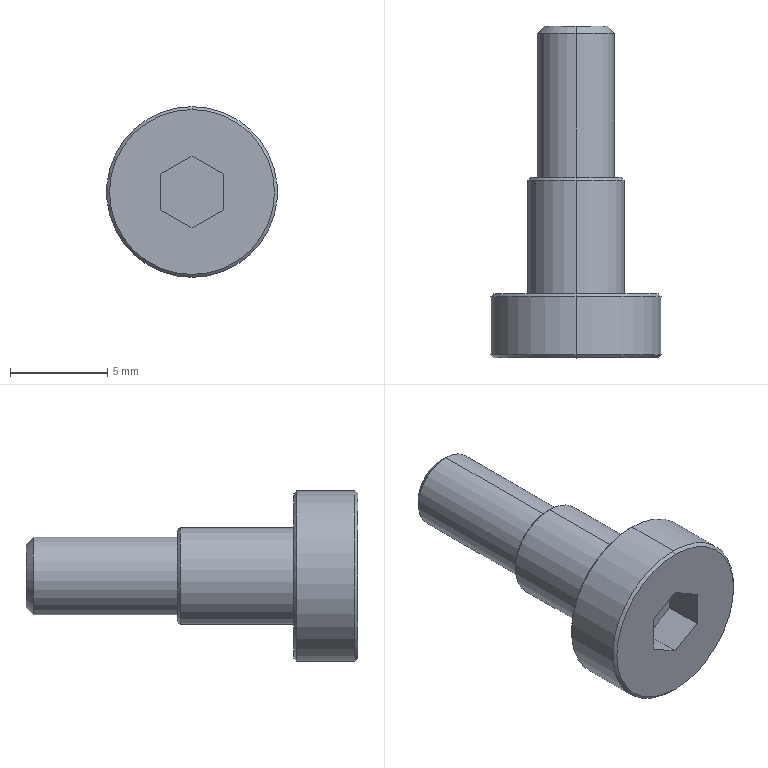Part | SolidWorks | features ICE 2, Chamfer 1, Extrusion 1, StudWizard 1 | 1 solid | 25 faces | box 8.8 x 17.1 x 8.8 mm | volume 397.168 mm3 | plane 11 | cone 8 | cylinder 6 | commonest cylinder face diameters 4 x2 5 x2 8.8 x2
STEP:
#1=CARTESIAN_POINT('',(0.,9.3,2.35));
#2=VERTEX_POINT('',#1);
#3=CARTESIAN_POINT('',(0.,9.3,-2.35));
#4=VERTEX_POINT('',#3);
#5=CARTESIAN_POINT('',(0.,9.3,0.));
#6=DIRECTION('',(0.,1.,0.));
#7=DIRECTION('',(0.,0.,1.));
#8=AXIS2_PLACEMENT_3D('',#5,#6,#7);
#9=CIRCLE('',#8,2.35);
#10=EDGE_CURVE('',#2,#4,#9,.T.);
#11=ORIENTED_EDGE('',*,*,#10,.F.);
#12=CARTESIAN_POINT('',(0.,9.15,2.5));
#13=VERTEX_POINT('',#12);
#14=CARTESIAN_POINT('',(0.,9.3,2.35));
#15=DIRECTION('',(0.,-0.7071,0.7071));
#16=VECTOR('',#15,1000.);
#17=LINE('',#14,#16);
#18=EDGE_CURVE('',#2,#13,#17,.T.);
#19=ORIENTED_EDGE('',*,*,#18,.T.);
#20=CARTESIAN_POINT('',(0.,9.15,-2.5));
#21=VERTEX_POINT('',#20);
#22=CARTESIAN_POINT('',(0.,9.15,0.));
#23=DIRECTION('',(0.,-1.,0.));
#24=DIRECTION('',(0.,0.,1.));
#25=AXIS2_PLACEMENT_3D('',#22,#23,#24);
#26=CIRCLE('',#25,2.5);
#27=EDGE_CURVE('',#21,#13,#26,.T.);
#28=ORIENTED_EDGE('',*,*,#27,.F.);
#29=CARTESIAN_POINT('',(0.,9.3,-2.35));
#30=DIRECTION('',(0.,-0.7071,-0.7071));
#31=VECTOR('',#30,1000.);
#32=LINE('',#29,#31);
#33=EDGE_CURVE('',#4,#21,#32,.T.);
#34=ORIENTED_EDGE('',*,*,#33,.F.);
#35=EDGE_LOOP('',(#11,#19,#28,#34));
#36=FACE_OUTER_BOUND('',#35,.T.);
#37=CARTESIAN_POINT('',(0.,9.3,0.));
#38=DIRECTION('',(0.,-1.,0.));
#39=DIRECTION('',(0.,0.,-1.));
#40=AXIS2_PLACEMENT_3D('',#37,#38,#39);
#41=CONICAL_SURFACE('',#40,2.35,0.7854);
#42=ADVANCED_FACE('',(#36),#41,.T.);
#43=CARTESIAN_POINT('',(0.,3.3,4.25));
#44=VERTEX_POINT('',#43);
#45=CARTESIAN_POINT('',(0.,3.3,-4.25));
#46=VERTEX_POINT('',#45);
#47=CARTESIAN_POINT('',(0.,3.3,0.));
#48=DIRECTION('',(0.,1.,0.));
#49=DIRECTION('',(0.,0.,1.));
#50=AXIS2_PLACEMENT_3D('',#47,#48,#49);
#51=CIRCLE('',#50,4.25);
#52=EDGE_CURVE('',#44,#46,#51,.T.);
#53=ORIENTED_EDGE('',*,*,#52,.F.);
#54=CARTESIAN_POINT('',(0.,3.15,4.4));
#55=VERTEX_POINT('',#54);
#56=CARTESIAN_POINT('',(0.,3.3,4.25));
#57=DIRECTION('',(0.,-0.7071,0.7071));
#58=VECTOR('',#57,1000.);
#59=LINE('',#56,#58);
#60=EDGE_CURVE('',#44,#55,#59,.T.);
#61=ORIENTED_EDGE('',*,*,#60,.T.);
#62=CARTESIAN_POINT('',(0.,3.15,-4.4));
#63=VERTEX_POINT('',#62);
#64=CARTESIAN_POINT('',(0.,3.15,0.));
#65=DIRECTION('',(0.,-1.,0.));
#66=DIRECTION('',(0.,0.,1.));
#67=AXIS2_PLACEMENT_3D('',#64,#65,#66);
#68=CIRCLE('',#67,4.4);
#69=EDGE_CURVE('',#63,#55,#68,.T.);
#70=ORIENTED_EDGE('',*,*,#69,.F.);
#71=CARTESIAN_POINT('',(0.,3.3,-4.25));
#72=DIRECTION('',(0.,-0.7071,-0.7071));
#73=VECTOR('',#72,1000.);
#74=LINE('',#71,#73);
#75=EDGE_CURVE('',#46,#63,#74,.T.);
#76=ORIENTED_EDGE('',*,*,#75,.F.);
#77=EDGE_LOOP('',(#53,#61,#70,#76));
#78=FACE_OUTER_BOUND('',#77,.T.);
#79=CARTESIAN_POINT('',(0.,3.3,0.));
#80=DIRECTION('',(0.,-1.,0.));
#81=DIRECTION('',(0.,0.,-1.));
#82=AXIS2_PLACEMENT_3D('',#79,#80,#81);
#83=CONICAL_SURFACE('',#82,4.25,0.7854);
#84=ADVANCED_FACE('',(#78),#83,.T.);
#85=CARTESIAN_POINT('',(0.,0.,-4.25));
#86=VERTEX_POINT('',#85);
#87=CARTESIAN_POINT('',(0.,0.,4.25));
#88=VERTEX_POINT('',#87);
#89=CARTESIAN_POINT('',(0.,0.,0.));
#90=DIRECTION('',(0.,-1.,0.));
#91=DIRECTION('',(0.,0.,1.));
#92=AXIS2_PLACEMENT_3D('',#89,#90,#91);
#93=CIRCLE('',#92,4.25);
#94=EDGE_CURVE('',#86,#88,#93,.T.);
#95=ORIENTED_EDGE('',*,*,#94,.F.);
#96=CARTESIAN_POINT('',(0.,0.15,-4.4));
#97=VERTEX_POINT('',#96);
#98=CARTESIAN_POINT('',(0.,0.15,-4.4));
#99=DIRECTION('',(0.,0.7071,-0.7071));
#100=VECTOR('',#99,1000.);
#101=LINE('',#98,#100);
#102=EDGE_CURVE('',#86,#97,#101,.T.);
#103=ORIENTED_EDGE('',*,*,#102,.T.);
#104=CARTESIAN_POINT('',(0.,0.15,4.4));
#105=VERTEX_POINT('',#104);
#106=CARTESIAN_POINT('',(0.,0.15,0.));
#107=DIRECTION('',(0.,1.,0.));
#108=DIRECTION('',(0.,0.,1.));
#109=AXIS2_PLACEMENT_3D('',#106,#107,#108);
#110=CIRCLE('',#109,4.4);
#111=EDGE_CURVE('',#105,#97,#110,.T.);
#112=ORIENTED_EDGE('',*,*,#111,.F.);
#113=CARTESIAN_POINT('',(0.,0.15,4.4));
#114=DIRECTION('',(0.,0.7071,0.7071));
#115=VECTOR('',#114,1000.);
#116=LINE('',#113,#115);
#117=EDGE_CURVE('',#88,#105,#116,.T.);
#118=ORIENTED_EDGE('',*,*,#117,.F.);
#119=EDGE_LOOP('',(#95,#103,#112,#118));
#120=FACE_OUTER_BOUND('',#119,.T.);
#121=CARTESIAN_POINT('',(0.,0.15,0.));
#122=DIRECTION('',(0.,1.,0.));
#123=DIRECTION('',(0.,0.,1.));
#124=AXIS2_PLACEMENT_3D('',#121,#122,#123);
#125=CONICAL_SURFACE('',#124,4.4,0.7854);
#126=ADVANCED_FACE('',(#120),#125,.T.);
#127=CARTESIAN_POINT('',(0.,16.721,-2.));
#128=VERTEX_POINT('',#127);
#129=CARTESIAN_POINT('',(0.,16.721,2.));
#130=VERTEX_POINT('',#129);
#131=CARTESIAN_POINT('',(0.,16.721,0.));
#132=DIRECTION('',(0.,-1.,0.));
#133=DIRECTION('',(0.,0.,-1.));
#134=AXIS2_PLACEMENT_3D('',#131,#132,#133);
#135=CIRCLE('',#134,2.);
#136=EDGE_CURVE('',#128,#130,#135,.T.);
#137=ORIENTED_EDGE('',*,*,#136,.T.);
#138=CARTESIAN_POINT('',(0.,9.3,2.));
#139=VERTEX_POINT('',#138);
#140=CARTESIAN_POINT('',(0.,9.3,2.));
#141=DIRECTION('',(0.,-1.,0.));
#142=VECTOR('',#141,1000.);
#143=LINE('',#140,#142);
#144=EDGE_CURVE('',#130,#139,#143,.T.);
#145=ORIENTED_EDGE('',*,*,#144,.T.);
#146=CARTESIAN_POINT('',(0.,9.3,-2.));
#147=VERTEX_POINT('',#146);
#148=CARTESIAN_POINT('',(0.,9.3,0.));
#149=DIRECTION('',(0.,-1.,0.));
#150=DIRECTION('',(0.,0.,-1.));
#151=AXIS2_PLACEMENT_3D('',#148,#149,#150);
#152=CIRCLE('',#151,2.);
#153=EDGE_CURVE('',#147,#139,#152,.T.);
#154=ORIENTED_EDGE('',*,*,#153,.F.);
#155=CARTESIAN_POINT('',(0.,9.3,-2.));
#156=DIRECTION('',(0.,-1.,0.));
#157=VECTOR('',#156,1000.);
#158=LINE('',#155,#157);
#159=EDGE_CURVE('',#128,#147,#158,.T.);
#160=ORIENTED_EDGE('',*,*,#159,.F.);
#161=EDGE_LOOP('',(#137,#145,#154,#160));
#162=FACE_OUTER_BOUND('',#161,.T.);
#163=CARTESIAN_POINT('',(0.,9.3,0.));
#164=DIRECTION('',(0.,-1.,0.));
#165=DIRECTION('',(0.,0.,-1.));
#166=AXIS2_PLACEMENT_3D('',#163,#164,#165);
#167=CYLINDRICAL_SURFACE('',#166,2.);
#168=ADVANCED_FACE('',(#162),#167,.T.);
#169=CARTESIAN_POINT('',(0.,17.1,-1.621));
#170=VERTEX_POINT('',#169);
#171=CARTESIAN_POINT('',(0.,17.1,1.621));
#172=VERTEX_POINT('',#171);
#173=CARTESIAN_POINT('',(0.,17.1,0.));
#174=DIRECTION('',(0.,-1.,0.));
#175=DIRECTION('',(0.,0.,-1.));
#176=AXIS2_PLACEMENT_3D('',#173,#174,#175);
#177=CIRCLE('',#176,1.621);
#178=EDGE_CURVE('',#170,#172,#177,.T.);
#179=ORIENTED_EDGE('',*,*,#178,.T.);
#180=CARTESIAN_POINT('',(0.,16.721,2.));
#181=DIRECTION('',(0.,-0.7071,0.7071));
#182=VECTOR('',#181,1000.);
#183=LINE('',#180,#182);
#184=EDGE_CURVE('',#172,#130,#183,.T.);
#185=ORIENTED_EDGE('',*,*,#184,.T.);
#186=ORIENTED_EDGE('',*,*,#136,.F.);
#187=CARTESIAN_POINT('',(0.,16.721,-2.));
#188=DIRECTION('',(0.,-0.7071,-0.7071));
#189=VECTOR('',#188,1000.);
#190=LINE('',#187,#189);
#191=EDGE_CURVE('',#170,#128,#190,.T.);
#192=ORIENTED_EDGE('',*,*,#191,.F.);
#193=EDGE_LOOP('',(#179,#185,#186,#192));
#194=FACE_OUTER_BOUND('',#193,.T.);
#195=CARTESIAN_POINT('',(0.,16.721,0.));
#196=DIRECTION('',(0.,-1.,0.));
#197=DIRECTION('',(0.,0.,-1.));
#198=AXIS2_PLACEMENT_3D('',#195,#196,#197);
#199=CONICAL_SURFACE('',#198,2.,0.7854);
#200=ADVANCED_FACE('',(#194),#199,.T.);
#201=ORIENTED_EDGE('',*,*,#27,.T.);
#202=CARTESIAN_POINT('',(0.,3.3,2.5));
#203=VERTEX_POINT('',#202);
#204=CARTESIAN_POINT('',(0.,9.3,2.5));
#205=DIRECTION('',(0.,-1.,0.));
#206=VECTOR('',#205,1000.);
#207=LINE('',#204,#206);
#208=EDGE_CURVE('',#13,#203,#207,.T.);
#209=ORIENTED_EDGE('',*,*,#208,.T.);
#210=CARTESIAN_POINT('',(0.,3.3,-2.5));
#211=VERTEX_POINT('',#210);
#212=CARTESIAN_POINT('',(0.,3.3,0.));
#213=DIRECTION('',(0.,1.,0.));
#214=DIRECTION('',(0.,0.,1.));
#215=AXIS2_PLACEMENT_3D('',#212,#213,#214);
#216=CIRCLE('',#215,2.5);
#217=EDGE_CURVE('',#203,#211,#216,.T.);
#218=ORIENTED_EDGE('',*,*,#217,.T.);
#219=CARTESIAN_POINT('',(0.,9.3,-2.5));
#220=DIRECTION('',(0.,-1.,0.));
#221=VECTOR('',#220,1000.);
#222=LINE('',#219,#221);
#223=EDGE_CURVE('',#21,#211,#222,.T.);
#224=ORIENTED_EDGE('',*,*,#223,.F.);
#225=EDGE_LOOP('',(#201,#209,#218,#224));
#226=FACE_OUTER_BOUND('',#225,.T.);
#227=CARTESIAN_POINT('',(0.,9.3,0.));
#228=DIRECTION('',(0.,-1.,0.));
#229=DIRECTION('',(0.,0.,-1.));
#230=AXIS2_PLACEMENT_3D('',#227,#228,#229);
#231=CYLINDRICAL_SURFACE('',#230,2.5);
#232=ADVANCED_FACE('',(#226),#231,.T.);
#233=ORIENTED_EDGE('',*,*,#69,.T.);
#234=CARTESIAN_POINT('',(0.,3.3,4.4));
#235=DIRECTION('',(0.,-1.,0.));
#236=VECTOR('',#235,1000.);
#237=LINE('',#234,#236);
#238=EDGE_CURVE('',#55,#105,#237,.T.);
#239=ORIENTED_EDGE('',*,*,#238,.T.);
#240=ORIENTED_EDGE('',*,*,#111,.T.);
#241=CARTESIAN_POINT('',(0.,3.3,-4.4));
#242=DIRECTION('',(0.,-1.,0.));
#243=VECTOR('',#242,1000.);
#244=LINE('',#241,#243);
#245=EDGE_CURVE('',#63,#97,#244,.T.);
#246=ORIENTED_EDGE('',*,*,#245,.F.);
#247=EDGE_LOOP('',(#233,#239,#240,#246));
#248=FACE_OUTER_BOUND('',#247,.T.);
#249=CARTESIAN_POINT('',(0.,3.3,0.));
#250=DIRECTION('',(0.,-1.,0.));
#251=DIRECTION('',(0.,0.,-1.));
#252=AXIS2_PLACEMENT_3D('',#249,#250,#251);
#253=CYLINDRICAL_SURFACE('',#252,4.4);
#254=ADVANCED_FACE('',(#248),#253,.T.);
#255=ORIENTED_EDGE('',*,*,#238,.F.);
#256=CARTESIAN_POINT('',(0.,3.15,0.));
#257=DIRECTION('',(0.,-1.,0.));
#258=DIRECTION('',(0.,0.,1.));
#259=AXIS2_PLACEMENT_3D('',#256,#257,#258);
#260=CIRCLE('',#259,4.4);
#261=EDGE_CURVE('',#55,#63,#260,.T.);
#262=ORIENTED_EDGE('',*,*,#261,.T.);
#263=ORIENTED_EDGE('',*,*,#245,.T.);
#264=CARTESIAN_POINT('',(0.,0.15,0.));
#265=DIRECTION('',(0.,1.,0.));
#266=DIRECTION('',(0.,0.,1.));
#267=AXIS2_PLACEMENT_3D('',#264,#265,#266);
#268=CIRCLE('',#267,4.4);
#269=EDGE_CURVE('',#97,#105,#268,.T.);
#270=ORIENTED_EDGE('',*,*,#269,.T.);
#271=EDGE_LOOP('',(#255,#262,#263,#270));
#272=FACE_OUTER_BOUND('',#271,.T.);
#273=CARTESIAN_POINT('',(0.,3.3,0.));
#274=DIRECTION('',(0.,-1.,0.));
#275=DIRECTION('',(0.,0.,-1.));
#276=AXIS2_PLACEMENT_3D('',#273,#274,#275);
#277=CYLINDRICAL_SURFACE('',#276,4.4);
#278=ADVANCED_FACE('',(#272),#277,.T.);
#279=CARTESIAN_POINT('',(0.,3.3,0.));
#280=DIRECTION('',(0.,1.,0.));
#281=DIRECTION('',(0.,0.,1.));
#282=AXIS2_PLACEMENT_3D('',#279,#280,#281);
#283=CIRCLE('',#282,4.25);
#284=EDGE_CURVE('',#46,#44,#283,.T.);
#285=ORIENTED_EDGE('',*,*,#284,.T.);
#286=ORIENTED_EDGE('',*,*,#52,.T.);
#287=EDGE_LOOP('',(#285,#286));
#288=FACE_OUTER_BOUND('',#287,.T.);
#289=CARTESIAN_POINT('',(0.,3.3,0.));
#290=DIRECTION('',(0.,1.,0.));
#291=DIRECTION('',(0.,0.,1.));
#292=AXIS2_PLACEMENT_3D('',#289,#290,#291);
#293=CIRCLE('',#292,2.5);
#294=EDGE_CURVE('',#211,#203,#293,.T.);
#295=ORIENTED_EDGE('',*,*,#294,.F.);
#296=ORIENTED_EDGE('',*,*,#217,.F.);
#297=EDGE_LOOP('',(#295,#296));
#298=FACE_BOUND('',#297,.T.);
#299=CARTESIAN_POINT('',(0.,3.3,0.));
#300=DIRECTION('',(0.,1.,0.));
#301=DIRECTION('',(0.,0.,1.));
#302=AXIS2_PLACEMENT_3D('',#299,#300,#301);
#303=PLANE('',#302);
#304=ADVANCED_FACE('',(#288,#298),#303,.T.);
#305=CARTESIAN_POINT('',(0.,0.,0.));
#306=DIRECTION('',(0.,-1.,0.));
#307=DIRECTION('',(0.,0.,1.));
#308=AXIS2_PLACEMENT_3D('',#305,#306,#307);
#309=CIRCLE('',#308,4.25);
#310=EDGE_CURVE('',#88,#86,#309,.T.);
#311=ORIENTED_EDGE('',*,*,#310,.T.);
#312=ORIENTED_EDGE('',*,*,#94,.T.);
#313=EDGE_LOOP('',(#311,#312));
#314=FACE_OUTER_BOUND('',#313,.T.);
#315=CARTESIAN_POINT('',(0.,0.,1.848));
#316=VERTEX_POINT('',#315);
#317=CARTESIAN_POINT('',(-1.6,0.,0.9238));
#318=VERTEX_POINT('',#317);
#319=CARTESIAN_POINT('',(0.,0.,1.848));
#320=DIRECTION('',(-0.866,0.,-0.5));
#321=VECTOR('',#320,1000.);
#322=LINE('',#319,#321);
#323=EDGE_CURVE('',#316,#318,#322,.T.);
#324=ORIENTED_EDGE('',*,*,#323,.F.);
#325=CARTESIAN_POINT('',(1.6,0.,0.9238));
#326=VERTEX_POINT('',#325);
#327=CARTESIAN_POINT('',(1.6,0.,0.9238));
#328=DIRECTION('',(-0.866,0.,0.5));
#329=VECTOR('',#328,1000.);
#330=LINE('',#327,#329);
#331=EDGE_CURVE('',#326,#316,#330,.T.);
#332=ORIENTED_EDGE('',*,*,#331,.F.);
#333=CARTESIAN_POINT('',(1.6,0.,-0.9238));
#334=VERTEX_POINT('',#333);
#335=CARTESIAN_POINT('',(1.6,0.,-0.9238));
#336=DIRECTION('',(0.,0.,1.));
#337=VECTOR('',#336,1000.);
#338=LINE('',#335,#337);
#339=EDGE_CURVE('',#334,#326,#338,.T.);
#340=ORIENTED_EDGE('',*,*,#339,.F.);
#341=CARTESIAN_POINT('',(0.,0.,-1.848));
#342=VERTEX_POINT('',#341);
#343=CARTESIAN_POINT('',(0.,0.,-1.848));
#344=DIRECTION('',(0.866,0.,0.5));
#345=VECTOR('',#344,1000.);
#346=LINE('',#343,#345);
#347=EDGE_CURVE('',#342,#334,#346,.T.);
#348=ORIENTED_EDGE('',*,*,#347,.F.);
#349=CARTESIAN_POINT('',(-1.6,0.,-0.9238));
#350=VERTEX_POINT('',#349);
#351=CARTESIAN_POINT('',(-1.6,0.,-0.9238));
#352=DIRECTION('',(0.866,0.,-0.5));
#353=VECTOR('',#352,1000.);
#354=LINE('',#351,#353);
#355=EDGE_CURVE('',#350,#342,#354,.T.);
#356=ORIENTED_EDGE('',*,*,#355,.F.);
#357=CARTESIAN_POINT('',(-1.6,0.,0.9238));
#358=DIRECTION('',(0.,0.,-1.));
#359=VECTOR('',#358,1000.);
#360=LINE('',#357,#359);
#361=EDGE_CURVE('',#318,#350,#360,.T.);
#362=ORIENTED_EDGE('',*,*,#361,.F.);
#363=EDGE_LOOP('',(#324,#332,#340,#348,#356,#362));
#364=FACE_BOUND('',#363,.T.);
#365=CARTESIAN_POINT('',(0.,0.,0.));
#366=DIRECTION('',(0.,1.,0.));
#367=DIRECTION('',(0.,0.,1.));
#368=AXIS2_PLACEMENT_3D('',#365,#366,#367);
#369=PLANE('',#368);
#370=ADVANCED_FACE('',(#314,#364),#369,.F.);
#371=ORIENTED_EDGE('',*,*,#208,.F.);
#372=CARTESIAN_POINT('',(0.,9.15,0.));
#373=DIRECTION('',(0.,-1.,0.));
#374=DIRECTION('',(0.,0.,1.));
#375=AXIS2_PLACEMENT_3D('',#372,#373,#374);
#376=CIRCLE('',#375,2.5);
#377=EDGE_CURVE('',#13,#21,#376,.T.);
#378=ORIENTED_EDGE('',*,*,#377,.T.);
#379=ORIENTED_EDGE('',*,*,#223,.T.);
#380=ORIENTED_EDGE('',*,*,#294,.T.);
#381=EDGE_LOOP('',(#371,#378,#379,#380));
#382=FACE_OUTER_BOUND('',#381,.T.);
#383=CARTESIAN_POINT('',(0.,9.3,0.));
#384=DIRECTION('',(0.,-1.,0.));
#385=DIRECTION('',(0.,0.,-1.));
#386=AXIS2_PLACEMENT_3D('',#383,#384,#385);
#387=CYLINDRICAL_SURFACE('',#386,2.5);
#388=ADVANCED_FACE('',(#382),#387,.T.);
#389=CARTESIAN_POINT('',(0.,9.3,0.));
#390=DIRECTION('',(0.,1.,0.));
#391=DIRECTION('',(0.,0.,1.));
#392=AXIS2_PLACEMENT_3D('',#389,#390,#391);
#393=CIRCLE('',#392,2.35);
#394=EDGE_CURVE('',#4,#2,#393,.T.);
#395=ORIENTED_EDGE('',*,*,#394,.T.);
#396=ORIENTED_EDGE('',*,*,#10,.T.);
#397=EDGE_LOOP('',(#395,#396));
#398=FACE_OUTER_BOUND('',#397,.T.);
#399=ORIENTED_EDGE('',*,*,#153,.T.);
#400=CARTESIAN_POINT('',(0.,9.3,0.));
#401=DIRECTION('',(0.,-1.,0.));
#402=DIRECTION('',(0.,0.,-1.));
#403=AXIS2_PLACEMENT_3D('',#400,#401,#402);
#404=CIRCLE('',#403,2.);
#405=EDGE_CURVE('',#139,#147,#404,.T.);
#406=ORIENTED_EDGE('',*,*,#405,.T.);
#407=EDGE_LOOP('',(#399,#406));
#408=FACE_BOUND('',#407,.T.);
#409=CARTESIAN_POINT('',(0.,9.3,0.));
#410=DIRECTION('',(0.,1.,0.));
#411=DIRECTION('',(0.,0.,1.));
#412=AXIS2_PLACEMENT_3D('',#409,#410,#411);
#413=PLANE('',#412);
#414=ADVANCED_FACE('',(#398,#408),#413,.T.);
#415=ORIENTED_EDGE('',*,*,#178,.F.);
#416=CARTESIAN_POINT('',(0.,17.1,0.));
#417=DIRECTION('',(0.,-1.,0.));
#418=DIRECTION('',(0.,0.,-1.));
#419=AXIS2_PLACEMENT_3D('',#416,#417,#418);
#420=CIRCLE('',#419,1.621);
#421=EDGE_CURVE('',#172,#170,#420,.T.);
#422=ORIENTED_EDGE('',*,*,#421,.F.);
#423=EDGE_LOOP('',(#415,#422));
#424=FACE_OUTER_BOUND('',#423,.T.);
#425=CARTESIAN_POINT('',(1.621,17.1,0.));
#426=DIRECTION('',(0.,1.,0.));
#427=DIRECTION('',(0.,0.,1.));
#428=AXIS2_PLACEMENT_3D('',#425,#426,#427);
#429=PLANE('',#428);
#430=ADVANCED_FACE('',(#424),#429,.T.);
#431=ORIENTED_EDGE('',*,*,#184,.F.);
#432=ORIENTED_EDGE('',*,*,#421,.T.);
#433=ORIENTED_EDGE('',*,*,#191,.T.);
#434=CARTESIAN_POINT('',(0.,16.721,0.));
#435=DIRECTION('',(0.,-1.,0.));
#436=DIRECTION('',(0.,0.,-1.));
#437=AXIS2_PLACEMENT_3D('',#434,#435,#436);
#438=CIRCLE('',#437,2.);
#439=EDGE_CURVE('',#130,#128,#438,.T.);
#440=ORIENTED_EDGE('',*,*,#439,.F.);
#441=EDGE_LOOP('',(#431,#432,#433,#440));
#442=FACE_OUTER_BOUND('',#441,.T.);
#443=CARTESIAN_POINT('',(0.,16.721,0.));
#444=DIRECTION('',(0.,-1.,0.));
#445=DIRECTION('',(0.,0.,-1.));
#446=AXIS2_PLACEMENT_3D('',#443,#444,#445);
#447=CONICAL_SURFACE('',#446,2.,0.7854);
#448=ADVANCED_FACE('',(#442),#447,.T.);
#449=ORIENTED_EDGE('',*,*,#144,.F.);
#450=ORIENTED_EDGE('',*,*,#439,.T.);
#451=ORIENTED_EDGE('',*,*,#159,.T.);
#452=ORIENTED_EDGE('',*,*,#405,.F.);
#453=EDGE_LOOP('',(#449,#450,#451,#452));
#454=FACE_OUTER_BOUND('',#453,.T.);
#455=CARTESIAN_POINT('',(0.,9.3,0.));
#456=DIRECTION('',(0.,-1.,0.));
#457=DIRECTION('',(0.,0.,-1.));
#458=AXIS2_PLACEMENT_3D('',#455,#456,#457);
#459=CYLINDRICAL_SURFACE('',#458,2.);
#460=ADVANCED_FACE('',(#454),#459,.T.);
#461=ORIENTED_EDGE('',*,*,#331,.T.);
#462=CARTESIAN_POINT('',(0.,2.,1.848));
#463=VERTEX_POINT('',#462);
#464=CARTESIAN_POINT('',(0.,2.,1.848));
#465=DIRECTION('',(0.,-1.,0.));
#466=VECTOR('',#465,1000.);
#467=LINE('',#464,#466);
#468=EDGE_CURVE('',#463,#316,#467,.T.);
#469=ORIENTED_EDGE('',*,*,#468,.F.);
#470=CARTESIAN_POINT('',(1.6,2.,0.9238));
#471=VERTEX_POINT('',#470);
#472=CARTESIAN_POINT('',(1.6,2.,0.9238));
#473=DIRECTION('',(-0.866,0.,0.5));
#474=VECTOR('',#473,1000.);
#475=LINE('',#472,#474);
#476=EDGE_CURVE('',#471,#463,#475,.T.);
#477=ORIENTED_EDGE('',*,*,#476,.F.);
#478=CARTESIAN_POINT('',(1.6,2.,0.9238));
#479=DIRECTION('',(0.,-1.,0.));
#480=VECTOR('',#479,1000.);
#481=LINE('',#478,#480);
#482=EDGE_CURVE('',#471,#326,#481,.T.);
#483=ORIENTED_EDGE('',*,*,#482,.T.);
#484=EDGE_LOOP('',(#461,#469,#477,#483));
#485=FACE_OUTER_BOUND('',#484,.T.);
#486=CARTESIAN_POINT('',(1.6,2.,0.9238));
#487=DIRECTION('',(0.5,0.,0.866));
#488=DIRECTION('',(0.866,0.,-0.5));
#489=AXIS2_PLACEMENT_3D('',#486,#487,#488);
#490=PLANE('',#489);
#491=ADVANCED_FACE('',(#485),#490,.F.);
#492=ORIENTED_EDGE('',*,*,#339,.T.);
#493=ORIENTED_EDGE('',*,*,#482,.F.);
#494=CARTESIAN_POINT('',(1.6,2.,-0.9238));
#495=VERTEX_POINT('',#494);
#496=CARTESIAN_POINT('',(1.6,2.,-0.9238));
#497=DIRECTION('',(0.,0.,1.));
#498=VECTOR('',#497,1000.);
#499=LINE('',#496,#498);
#500=EDGE_CURVE('',#495,#471,#499,.T.);
#501=ORIENTED_EDGE('',*,*,#500,.F.);
#502=CARTESIAN_POINT('',(1.6,2.,-0.9238));
#503=DIRECTION('',(0.,-1.,0.));
#504=VECTOR('',#503,1000.);
#505=LINE('',#502,#504);
#506=EDGE_CURVE('',#495,#334,#505,.T.);
#507=ORIENTED_EDGE('',*,*,#506,.T.);
#508=EDGE_LOOP('',(#492,#493,#501,#507));
#509=FACE_OUTER_BOUND('',#508,.T.);
#510=CARTESIAN_POINT('',(1.6,2.,-0.9238));
#511=DIRECTION('',(1.,0.,0.));
#512=DIRECTION('',(0.,0.,-1.));
#513=AXIS2_PLACEMENT_3D('',#510,#511,#512);
#514=PLANE('',#513);
#515=ADVANCED_FACE('',(#509),#514,.F.);
#516=ORIENTED_EDGE('',*,*,#347,.T.);
#517=ORIENTED_EDGE('',*,*,#506,.F.);
#518=CARTESIAN_POINT('',(0.,2.,-1.848));
#519=VERTEX_POINT('',#518);
#520=CARTESIAN_POINT('',(0.,2.,-1.848));
#521=DIRECTION('',(0.866,0.,0.5));
#522=VECTOR('',#521,1000.);
#523=LINE('',#520,#522);
#524=EDGE_CURVE('',#519,#495,#523,.T.);
#525=ORIENTED_EDGE('',*,*,#524,.F.);
#526=CARTESIAN_POINT('',(0.,2.,-1.848));
#527=DIRECTION('',(0.,-1.,0.));
#528=VECTOR('',#527,1000.);
#529=LINE('',#526,#528);
#530=EDGE_CURVE('',#519,#342,#529,.T.);
#531=ORIENTED_EDGE('',*,*,#530,.T.);
#532=EDGE_LOOP('',(#516,#517,#525,#531));
#533=FACE_OUTER_BOUND('',#532,.T.);
#534=CARTESIAN_POINT('',(0.,2.,-1.848));
#535=DIRECTION('',(0.5,0.,-0.866));
#536=DIRECTION('',(-0.866,0.,-0.5));
#537=AXIS2_PLACEMENT_3D('',#534,#535,#536);
#538=PLANE('',#537);
#539=ADVANCED_FACE('',(#533),#538,.F.);
#540=ORIENTED_EDGE('',*,*,#355,.T.);
#541=ORIENTED_EDGE('',*,*,#530,.F.);
#542=CARTESIAN_POINT('',(-1.6,2.,-0.9238));
#543=VERTEX_POINT('',#542);
#544=CARTESIAN_POINT('',(-1.6,2.,-0.9238));
#545=DIRECTION('',(0.866,0.,-0.5));
#546=VECTOR('',#545,1000.);
#547=LINE('',#544,#546);
#548=EDGE_CURVE('',#543,#519,#547,.T.);
#549=ORIENTED_EDGE('',*,*,#548,.F.);
#550=CARTESIAN_POINT('',(-1.6,2.,-0.9238));
#551=DIRECTION('',(0.,-1.,0.));
#552=VECTOR('',#551,1000.);
#553=LINE('',#550,#552);
#554=EDGE_CURVE('',#543,#350,#553,.T.);
#555=ORIENTED_EDGE('',*,*,#554,.T.);
#556=EDGE_LOOP('',(#540,#541,#549,#555));
#557=FACE_OUTER_BOUND('',#556,.T.);
#558=CARTESIAN_POINT('',(-1.6,2.,-0.9238));
#559=DIRECTION('',(-0.5,0.,-0.866));
#560=DIRECTION('',(-0.866,0.,0.5));
#561=AXIS2_PLACEMENT_3D('',#558,#559,#560);
#562=PLANE('',#561);
#563=ADVANCED_FACE('',(#557),#562,.F.);
#564=ORIENTED_EDGE('',*,*,#361,.T.);
#565=ORIENTED_EDGE('',*,*,#554,.F.);
#566=CARTESIAN_POINT('',(-1.6,2.,0.9238));
#567=VERTEX_POINT('',#566);
#568=CARTESIAN_POINT('',(-1.6,2.,0.9238));
#569=DIRECTION('',(0.,0.,-1.));
#570=VECTOR('',#569,1000.);
#571=LINE('',#568,#570);
#572=EDGE_CURVE('',#567,#543,#571,.T.);
#573=ORIENTED_EDGE('',*,*,#572,.F.);
#574=CARTESIAN_POINT('',(-1.6,2.,0.9238));
#575=DIRECTION('',(0.,-1.,0.));
#576=VECTOR('',#575,1000.);
#577=LINE('',#574,#576);
#578=EDGE_CURVE('',#567,#318,#577,.T.);
#579=ORIENTED_EDGE('',*,*,#578,.T.);
#580=EDGE_LOOP('',(#564,#565,#573,#579));
#581=FACE_OUTER_BOUND('',#580,.T.);
#582=CARTESIAN_POINT('',(-1.6,2.,0.9238));
#583=DIRECTION('',(-1.,0.,0.));
#584=DIRECTION('',(0.,0.,1.));
#585=AXIS2_PLACEMENT_3D('',#582,#583,#584);
#586=PLANE('',#585);
#587=ADVANCED_FACE('',(#581),#586,.F.);
#588=ORIENTED_EDGE('',*,*,#323,.T.);
#589=ORIENTED_EDGE('',*,*,#578,.F.);
#590=CARTESIAN_POINT('',(0.,2.,1.848));
#591=DIRECTION('',(-0.866,0.,-0.5));
#592=VECTOR('',#591,1000.);
#593=LINE('',#590,#592);
#594=EDGE_CURVE('',#463,#567,#593,.T.);
#595=ORIENTED_EDGE('',*,*,#594,.F.);
#596=ORIENTED_EDGE('',*,*,#468,.T.);
#597=EDGE_LOOP('',(#588,#589,#595,#596));
#598=FACE_OUTER_BOUND('',#597,.T.);
#599=CARTESIAN_POINT('',(0.,2.,1.848));
#600=DIRECTION('',(-0.5,0.,0.866));
#601=DIRECTION('',(0.866,0.,0.5));
#602=AXIS2_PLACEMENT_3D('',#599,#600,#601);
#603=PLANE('',#602);
#604=ADVANCED_FACE('',(#598),#603,.F.);
#605=ORIENTED_EDGE('',*,*,#476,.T.);
#606=ORIENTED_EDGE('',*,*,#594,.T.);
#607=ORIENTED_EDGE('',*,*,#572,.T.);
#608=ORIENTED_EDGE('',*,*,#548,.T.);
#609=ORIENTED_EDGE('',*,*,#524,.T.);
#610=ORIENTED_EDGE('',*,*,#500,.T.);
#611=EDGE_LOOP('',(#605,#606,#607,#608,#609,#610));
#612=FACE_OUTER_BOUND('',#611,.T.);
#613=CARTESIAN_POINT('',(0.,2.,0.));
#614=DIRECTION('',(0.,-1.,0.));
#615=DIRECTION('',(0.,0.,-1.));
#616=AXIS2_PLACEMENT_3D('',#613,#614,#615);
#617=PLANE('',#616);
#618=ADVANCED_FACE('',(#612),#617,.T.);
#619=ORIENTED_EDGE('',*,*,#102,.F.);
#620=ORIENTED_EDGE('',*,*,#310,.F.);
#621=ORIENTED_EDGE('',*,*,#117,.T.);
#622=ORIENTED_EDGE('',*,*,#269,.F.);
#623=EDGE_LOOP('',(#619,#620,#621,#622));
#624=FACE_OUTER_BOUND('',#623,.T.);
#625=CARTESIAN_POINT('',(0.,0.15,0.));
#626=DIRECTION('',(0.,1.,0.));
#627=DIRECTION('',(0.,0.,1.));
#628=AXIS2_PLACEMENT_3D('',#625,#626,#627);
#629=CONICAL_SURFACE('',#628,4.4,0.7854);
#630=ADVANCED_FACE('',(#624),#629,.T.);
#631=ORIENTED_EDGE('',*,*,#60,.F.);
#632=ORIENTED_EDGE('',*,*,#284,.F.);
#633=ORIENTED_EDGE('',*,*,#75,.T.);
#634=ORIENTED_EDGE('',*,*,#261,.F.);
#635=EDGE_LOOP('',(#631,#632,#633,#634));
#636=FACE_OUTER_BOUND('',#635,.T.);
#637=CARTESIAN_POINT('',(0.,3.3,0.));
#638=DIRECTION('',(0.,-1.,0.));
#639=DIRECTION('',(0.,0.,-1.));
#640=AXIS2_PLACEMENT_3D('',#637,#638,#639);
#641=CONICAL_SURFACE('',#640,4.25,0.7854);
#642=ADVANCED_FACE('',(#636),#641,.T.);
#643=ORIENTED_EDGE('',*,*,#18,.F.);
#644=ORIENTED_EDGE('',*,*,#394,.F.);
#645=ORIENTED_EDGE('',*,*,#33,.T.);
#646=ORIENTED_EDGE('',*,*,#377,.F.);
#647=EDGE_LOOP('',(#643,#644,#645,#646));
#648=FACE_OUTER_BOUND('',#647,.T.);
#649=CARTESIAN_POINT('',(0.,9.3,0.));
#650=DIRECTION('',(0.,-1.,0.));
#651=DIRECTION('',(0.,0.,-1.));
#652=AXIS2_PLACEMENT_3D('',#649,#650,#651);
#653=CONICAL_SURFACE('',#652,2.35,0.7854);
#654=ADVANCED_FACE('',(#648),#653,.T.);
#655=CLOSED_SHELL('',(#42,#84,#126,#168,#200,#232,#254,#278,#304,#370,#388,#414,#430,#448,#460,#491,#515,#539,#563,#587,#604,#618,#630,#642,#654));
#656=MANIFOLD_SOLID_BREP('',#655);
#657=CARTESIAN_POINT('',(0.,0.,0.));
#658=DIRECTION('',(0.,0.,1.));
#659=DIRECTION('',(1.,0.,0.));
#660=AXIS2_PLACEMENT_3D('',#657,#658,#659);
#661=(LENGTH_UNIT()NAMED_UNIT(*)SI_UNIT(.MILLI.,.METRE.));
#662=UNCERTAINTY_MEASURE_WITH_UNIT(LENGTH_MEASURE(0.00001),#661,'','');
#663=(NAMED_UNIT(*)PLANE_ANGLE_UNIT()SI_UNIT($,.RADIAN.));
#664=(NAMED_UNIT(*)SI_UNIT($,.STERADIAN.)SOLID_ANGLE_UNIT());
#665=(GEOMETRIC_REPRESENTATION_CONTEXT(3)GLOBAL_UNCERTAINTY_ASSIGNED_CONTEXT((#662))GLOBAL_UNIT_ASSIGNED_CONTEXT((#661,#663,#664))REPRESENTATION_CONTEXT('',''));
#666=ADVANCED_BREP_SHAPE_REPRESENTATION('',(#656,#660),#665);